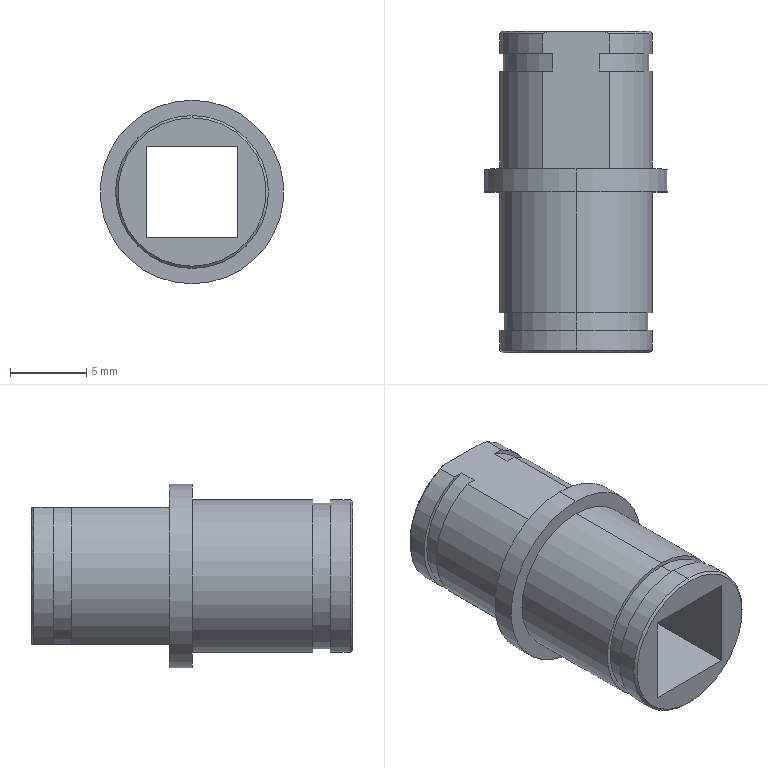Part | NX | features BREP 1 | 1 solid | 34 faces | box 12 x 21 x 12 mm | volume 902.734 mm3 | plane 16 | cylinder 14 | cone 4 | commonest cylinder face diameters 10 x8 9.5 x4 12 x2
STEP:
#1=CARTESIAN_POINT('',(0.,0.15,-5.));
#2=VERTEX_POINT('',#1);
#3=CARTESIAN_POINT('',(0.,0.,-4.85));
#4=VERTEX_POINT('',#3);
#5=CARTESIAN_POINT('',(0.,0.,-4.85));
#6=DIRECTION('',(0.,0.7071,-0.7071));
#7=VECTOR('',#6,1000.);
#8=LINE('',#5,#7);
#9=EDGE_CURVE('',#2,#4,#8,.F.);
#10=ORIENTED_EDGE('',*,*,#9,.T.);
#11=CARTESIAN_POINT('',(0.,0.,4.85));
#12=VERTEX_POINT('',#11);
#13=CARTESIAN_POINT('',(0.,0.,0.));
#14=DIRECTION('',(0.,-1.,0.));
#15=DIRECTION('',(0.,0.,1.));
#16=AXIS2_PLACEMENT_3D('',#13,#14,#15);
#17=CIRCLE('',#16,4.85);
#18=EDGE_CURVE('',#12,#4,#17,.T.);
#19=ORIENTED_EDGE('',*,*,#18,.F.);
#20=CARTESIAN_POINT('',(0.,0.15,5.));
#21=VERTEX_POINT('',#20);
#22=CARTESIAN_POINT('',(0.,0.,4.85));
#23=DIRECTION('',(0.,0.7071,0.7071));
#24=VECTOR('',#23,1000.);
#25=LINE('',#22,#24);
#26=EDGE_CURVE('',#21,#12,#25,.F.);
#27=ORIENTED_EDGE('',*,*,#26,.F.);
#28=CARTESIAN_POINT('',(0.,0.15,0.));
#29=DIRECTION('',(0.,1.,0.));
#30=DIRECTION('',(0.,0.,1.));
#31=AXIS2_PLACEMENT_3D('',#28,#29,#30);
#32=CIRCLE('',#31,5.);
#33=EDGE_CURVE('',#2,#21,#32,.T.);
#34=ORIENTED_EDGE('',*,*,#33,.F.);
#35=EDGE_LOOP('',(#10,#19,#27,#34));
#36=FACE_BOUND('',#35,.T.);
#37=CARTESIAN_POINT('',(0.,0.,0.));
#38=DIRECTION('',(0.,1.,0.));
#39=DIRECTION('',(0.,0.,1.));
#40=AXIS2_PLACEMENT_3D('',#37,#38,#39);
#41=CONICAL_SURFACE('',#40,4.85,0.7854);
#42=ADVANCED_FACE('',(#36),#41,.T.);
#43=CARTESIAN_POINT('',(1.809,21.,-4.5));
#44=VERTEX_POINT('',#43);
#45=CARTESIAN_POINT('',(2.179,20.85,-4.5));
#46=VERTEX_POINT('',#45);
#47=CARTESIAN_POINT('',(1.809,21.,-4.5));
#48=CARTESIAN_POINT('',(1.934,20.953,-4.5));
#49=CARTESIAN_POINT('',(2.057,20.903,-4.5));
#50=CARTESIAN_POINT('',(2.179,20.85,-4.5));
#51=B_SPLINE_CURVE_WITH_KNOTS('',3,(#47,#48,#49,#50),.UNSPECIFIED.,.F.,.F.,(4,4),(0.,0.0003997),.UNSPECIFIED.);
#52=EDGE_CURVE('',#44,#46,#51,.T.);
#53=ORIENTED_EDGE('',*,*,#52,.F.);
#54=CARTESIAN_POINT('',(1.809,21.,4.5));
#55=VERTEX_POINT('',#54);
#56=CARTESIAN_POINT('',(0.,21.,0.));
#57=DIRECTION('',(0.,1.,0.));
#58=DIRECTION('',(0.,0.,-1.));
#59=AXIS2_PLACEMENT_3D('',#56,#57,#58);
#60=CIRCLE('',#59,4.85);
#61=EDGE_CURVE('',#55,#44,#60,.T.);
#62=ORIENTED_EDGE('',*,*,#61,.F.);
#63=CARTESIAN_POINT('',(2.179,20.85,4.5));
#64=VERTEX_POINT('',#63);
#65=CARTESIAN_POINT('',(2.179,20.85,4.5));
#66=CARTESIAN_POINT('',(2.057,20.903,4.5));
#67=CARTESIAN_POINT('',(1.934,20.953,4.5));
#68=CARTESIAN_POINT('',(1.809,21.,4.5));
#69=B_SPLINE_CURVE_WITH_KNOTS('',3,(#65,#66,#67,#68),.UNSPECIFIED.,.F.,.F.,(4,4),(0.,0.0003997),.UNSPECIFIED.);
#70=EDGE_CURVE('',#64,#55,#69,.T.);
#71=ORIENTED_EDGE('',*,*,#70,.F.);
#72=CARTESIAN_POINT('',(0.,20.85,0.));
#73=DIRECTION('',(0.,-1.,0.));
#74=DIRECTION('',(0.,0.,-1.));
#75=AXIS2_PLACEMENT_3D('',#72,#73,#74);
#76=CIRCLE('',#75,5.);
#77=EDGE_CURVE('',#46,#64,#76,.T.);
#78=ORIENTED_EDGE('',*,*,#77,.F.);
#79=EDGE_LOOP('',(#53,#62,#71,#78));
#80=FACE_BOUND('',#79,.T.);
#81=CARTESIAN_POINT('',(0.,20.85,0.));
#82=DIRECTION('',(0.,-1.,0.));
#83=DIRECTION('',(0.,0.,-1.));
#84=AXIS2_PLACEMENT_3D('',#81,#82,#83);
#85=CONICAL_SURFACE('',#84,5.,0.7854);
#86=ADVANCED_FACE('',(#80),#85,.T.);
#87=CARTESIAN_POINT('',(-1.809,21.,4.5));
#88=VERTEX_POINT('',#87);
#89=CARTESIAN_POINT('',(-2.179,20.85,4.5));
#90=VERTEX_POINT('',#89);
#91=CARTESIAN_POINT('',(-1.809,21.,4.5));
#92=CARTESIAN_POINT('',(-1.934,20.953,4.5));
#93=CARTESIAN_POINT('',(-2.057,20.903,4.5));
#94=CARTESIAN_POINT('',(-2.179,20.85,4.5));
#95=B_SPLINE_CURVE_WITH_KNOTS('',3,(#91,#92,#93,#94),.UNSPECIFIED.,.F.,.F.,(4,4),(0.,0.0003997),.UNSPECIFIED.);
#96=EDGE_CURVE('',#88,#90,#95,.T.);
#97=ORIENTED_EDGE('',*,*,#96,.F.);
#98=CARTESIAN_POINT('',(-1.809,21.,-4.5));
#99=VERTEX_POINT('',#98);
#100=CARTESIAN_POINT('',(0.,21.,0.));
#101=DIRECTION('',(0.,1.,0.));
#102=DIRECTION('',(0.,0.,-1.));
#103=AXIS2_PLACEMENT_3D('',#100,#101,#102);
#104=CIRCLE('',#103,4.85);
#105=EDGE_CURVE('',#99,#88,#104,.T.);
#106=ORIENTED_EDGE('',*,*,#105,.F.);
#107=CARTESIAN_POINT('',(-2.179,20.85,-4.5));
#108=VERTEX_POINT('',#107);
#109=CARTESIAN_POINT('',(-2.179,20.85,-4.5));
#110=CARTESIAN_POINT('',(-2.057,20.903,-4.5));
#111=CARTESIAN_POINT('',(-1.934,20.953,-4.5));
#112=CARTESIAN_POINT('',(-1.809,21.,-4.5));
#113=B_SPLINE_CURVE_WITH_KNOTS('',3,(#109,#110,#111,#112),.UNSPECIFIED.,.F.,.F.,(4,4),(0.,0.0003997),.UNSPECIFIED.);
#114=EDGE_CURVE('',#108,#99,#113,.T.);
#115=ORIENTED_EDGE('',*,*,#114,.F.);
#116=CARTESIAN_POINT('',(0.,20.85,0.));
#117=DIRECTION('',(0.,-1.,0.));
#118=DIRECTION('',(0.,0.,-1.));
#119=AXIS2_PLACEMENT_3D('',#116,#117,#118);
#120=CIRCLE('',#119,5.);
#121=EDGE_CURVE('',#90,#108,#120,.T.);
#122=ORIENTED_EDGE('',*,*,#121,.F.);
#123=EDGE_LOOP('',(#97,#106,#115,#122));
#124=FACE_BOUND('',#123,.T.);
#125=CARTESIAN_POINT('',(0.,20.85,0.));
#126=DIRECTION('',(0.,-1.,0.));
#127=DIRECTION('',(0.,0.,-1.));
#128=AXIS2_PLACEMENT_3D('',#125,#126,#127);
#129=CONICAL_SURFACE('',#128,5.,0.7854);
#130=ADVANCED_FACE('',(#124),#129,.T.);
#131=CARTESIAN_POINT('',(-2.179,19.55,-4.5));
#132=VERTEX_POINT('',#131);
#133=CARTESIAN_POINT('',(-2.179,7.37,-4.5));
#134=DIRECTION('',(0.,1.,0.));
#135=VECTOR('',#134,1000.);
#136=LINE('',#133,#135);
#137=EDGE_CURVE('',#132,#108,#136,.T.);
#138=ORIENTED_EDGE('',*,*,#137,.T.);
#139=ORIENTED_EDGE('',*,*,#114,.T.);
#140=CARTESIAN_POINT('',(2.179,21.,-4.5));
#141=DIRECTION('',(1.,0.,0.));
#142=VECTOR('',#141,1000.);
#143=LINE('',#140,#142);
#144=EDGE_CURVE('',#99,#44,#143,.T.);
#145=ORIENTED_EDGE('',*,*,#144,.T.);
#146=ORIENTED_EDGE('',*,*,#52,.T.);
#147=CARTESIAN_POINT('',(2.179,19.55,-4.5));
#148=VERTEX_POINT('',#147);
#149=CARTESIAN_POINT('',(2.179,7.37,-4.5));
#150=DIRECTION('',(0.,1.,0.));
#151=VECTOR('',#150,1000.);
#152=LINE('',#149,#151);
#153=EDGE_CURVE('',#148,#46,#152,.T.);
#154=ORIENTED_EDGE('',*,*,#153,.F.);
#155=CARTESIAN_POINT('',(1.521,19.55,-4.5));
#156=VERTEX_POINT('',#155);
#157=CARTESIAN_POINT('',(0.,19.55,-4.5));
#158=DIRECTION('',(1.,0.,0.));
#159=VECTOR('',#158,1000.);
#160=LINE('',#157,#159);
#161=EDGE_CURVE('',#156,#148,#160,.T.);
#162=ORIENTED_EDGE('',*,*,#161,.F.);
#163=CARTESIAN_POINT('',(1.521,18.4,-4.5));
#164=VERTEX_POINT('',#163);
#165=CARTESIAN_POINT('',(1.521,19.55,-4.5));
#166=DIRECTION('',(0.,1.,0.));
#167=VECTOR('',#166,1000.);
#168=LINE('',#165,#167);
#169=EDGE_CURVE('',#164,#156,#168,.T.);
#170=ORIENTED_EDGE('',*,*,#169,.F.);
#171=CARTESIAN_POINT('',(2.179,18.4,-4.5));
#172=VERTEX_POINT('',#171);
#173=CARTESIAN_POINT('',(0.,18.4,-4.5));
#174=DIRECTION('',(1.,0.,0.));
#175=VECTOR('',#174,1000.);
#176=LINE('',#173,#175);
#177=EDGE_CURVE('',#164,#172,#176,.T.);
#178=ORIENTED_EDGE('',*,*,#177,.T.);
#179=CARTESIAN_POINT('',(2.179,12.,-4.5));
#180=VERTEX_POINT('',#179);
#181=CARTESIAN_POINT('',(2.179,7.37,-4.5));
#182=DIRECTION('',(0.,1.,0.));
#183=VECTOR('',#182,1000.);
#184=LINE('',#181,#183);
#185=EDGE_CURVE('',#180,#172,#184,.T.);
#186=ORIENTED_EDGE('',*,*,#185,.F.);
#187=CARTESIAN_POINT('',(-2.179,12.,-4.5));
#188=VERTEX_POINT('',#187);
#189=CARTESIAN_POINT('',(2.179,12.,-4.5));
#190=DIRECTION('',(1.,0.,0.));
#191=VECTOR('',#190,1000.);
#192=LINE('',#189,#191);
#193=EDGE_CURVE('',#188,#180,#192,.T.);
#194=ORIENTED_EDGE('',*,*,#193,.F.);
#195=CARTESIAN_POINT('',(-2.179,18.4,-4.5));
#196=VERTEX_POINT('',#195);
#197=CARTESIAN_POINT('',(-2.179,7.37,-4.5));
#198=DIRECTION('',(0.,1.,0.));
#199=VECTOR('',#198,1000.);
#200=LINE('',#197,#199);
#201=EDGE_CURVE('',#188,#196,#200,.T.);
#202=ORIENTED_EDGE('',*,*,#201,.T.);
#203=CARTESIAN_POINT('',(-1.521,18.4,-4.5));
#204=VERTEX_POINT('',#203);
#205=CARTESIAN_POINT('',(0.,18.4,-4.5));
#206=DIRECTION('',(1.,0.,0.));
#207=VECTOR('',#206,1000.);
#208=LINE('',#205,#207);
#209=EDGE_CURVE('',#196,#204,#208,.T.);
#210=ORIENTED_EDGE('',*,*,#209,.T.);
#211=CARTESIAN_POINT('',(-1.521,19.55,-4.5));
#212=VERTEX_POINT('',#211);
#213=CARTESIAN_POINT('',(-1.521,19.55,-4.5));
#214=DIRECTION('',(0.,-1.,0.));
#215=VECTOR('',#214,1000.);
#216=LINE('',#213,#215);
#217=EDGE_CURVE('',#212,#204,#216,.T.);
#218=ORIENTED_EDGE('',*,*,#217,.F.);
#219=CARTESIAN_POINT('',(0.,19.55,-4.5));
#220=DIRECTION('',(1.,0.,0.));
#221=VECTOR('',#220,1000.);
#222=LINE('',#219,#221);
#223=EDGE_CURVE('',#132,#212,#222,.T.);
#224=ORIENTED_EDGE('',*,*,#223,.F.);
#225=EDGE_LOOP('',(#138,#139,#145,#146,#154,#162,#170,#178,#186,#194,#202,#210,#218,#224));
#226=FACE_BOUND('',#225,.T.);
#227=CARTESIAN_POINT('',(2.179,7.37,-4.5));
#228=DIRECTION('',(0.,0.,1.));
#229=DIRECTION('',(1.,0.,0.));
#230=AXIS2_PLACEMENT_3D('',#227,#228,#229);
#231=PLANE('',#230);
#232=ADVANCED_FACE('',(#226),#231,.F.);
#233=CARTESIAN_POINT('',(2.179,21.,4.5));
#234=DIRECTION('',(-1.,0.,0.));
#235=VECTOR('',#234,1000.);
#236=LINE('',#233,#235);
#237=EDGE_CURVE('',#55,#88,#236,.T.);
#238=ORIENTED_EDGE('',*,*,#237,.T.);
#239=ORIENTED_EDGE('',*,*,#96,.T.);
#240=CARTESIAN_POINT('',(-2.179,19.55,4.5));
#241=VERTEX_POINT('',#240);
#242=CARTESIAN_POINT('',(-2.179,7.37,4.5));
#243=DIRECTION('',(0.,1.,0.));
#244=VECTOR('',#243,1000.);
#245=LINE('',#242,#244);
#246=EDGE_CURVE('',#241,#90,#245,.T.);
#247=ORIENTED_EDGE('',*,*,#246,.F.);
#248=CARTESIAN_POINT('',(-1.521,19.55,4.5));
#249=VERTEX_POINT('',#248);
#250=CARTESIAN_POINT('',(0.,19.55,4.5));
#251=DIRECTION('',(-1.,0.,0.));
#252=VECTOR('',#251,1000.);
#253=LINE('',#250,#252);
#254=EDGE_CURVE('',#249,#241,#253,.T.);
#255=ORIENTED_EDGE('',*,*,#254,.F.);
#256=CARTESIAN_POINT('',(-1.521,18.4,4.5));
#257=VERTEX_POINT('',#256);
#258=CARTESIAN_POINT('',(-1.521,19.55,4.5));
#259=DIRECTION('',(0.,1.,0.));
#260=VECTOR('',#259,1000.);
#261=LINE('',#258,#260);
#262=EDGE_CURVE('',#257,#249,#261,.T.);
#263=ORIENTED_EDGE('',*,*,#262,.F.);
#264=CARTESIAN_POINT('',(-2.179,18.4,4.5));
#265=VERTEX_POINT('',#264);
#266=CARTESIAN_POINT('',(0.,18.4,4.5));
#267=DIRECTION('',(-1.,0.,0.));
#268=VECTOR('',#267,1000.);
#269=LINE('',#266,#268);
#270=EDGE_CURVE('',#257,#265,#269,.T.);
#271=ORIENTED_EDGE('',*,*,#270,.T.);
#272=CARTESIAN_POINT('',(-2.179,12.,4.5));
#273=VERTEX_POINT('',#272);
#274=CARTESIAN_POINT('',(-2.179,7.37,4.5));
#275=DIRECTION('',(0.,1.,0.));
#276=VECTOR('',#275,1000.);
#277=LINE('',#274,#276);
#278=EDGE_CURVE('',#273,#265,#277,.T.);
#279=ORIENTED_EDGE('',*,*,#278,.F.);
#280=CARTESIAN_POINT('',(2.179,12.,4.5));
#281=VERTEX_POINT('',#280);
#282=CARTESIAN_POINT('',(2.179,12.,4.5));
#283=DIRECTION('',(-1.,0.,0.));
#284=VECTOR('',#283,1000.);
#285=LINE('',#282,#284);
#286=EDGE_CURVE('',#281,#273,#285,.T.);
#287=ORIENTED_EDGE('',*,*,#286,.F.);
#288=CARTESIAN_POINT('',(2.179,18.4,4.5));
#289=VERTEX_POINT('',#288);
#290=CARTESIAN_POINT('',(2.179,7.37,4.5));
#291=DIRECTION('',(0.,1.,0.));
#292=VECTOR('',#291,1000.);
#293=LINE('',#290,#292);
#294=EDGE_CURVE('',#281,#289,#293,.T.);
#295=ORIENTED_EDGE('',*,*,#294,.T.);
#296=CARTESIAN_POINT('',(1.521,18.4,4.5));
#297=VERTEX_POINT('',#296);
#298=CARTESIAN_POINT('',(0.,18.4,4.5));
#299=DIRECTION('',(-1.,0.,0.));
#300=VECTOR('',#299,1000.);
#301=LINE('',#298,#300);
#302=EDGE_CURVE('',#289,#297,#301,.T.);
#303=ORIENTED_EDGE('',*,*,#302,.T.);
#304=CARTESIAN_POINT('',(1.521,19.55,4.5));
#305=VERTEX_POINT('',#304);
#306=CARTESIAN_POINT('',(1.521,19.55,4.5));
#307=DIRECTION('',(0.,-1.,0.));
#308=VECTOR('',#307,1000.);
#309=LINE('',#306,#308);
#310=EDGE_CURVE('',#305,#297,#309,.T.);
#311=ORIENTED_EDGE('',*,*,#310,.F.);
#312=CARTESIAN_POINT('',(2.179,19.55,4.5));
#313=VERTEX_POINT('',#312);
#314=CARTESIAN_POINT('',(0.,19.55,4.5));
#315=DIRECTION('',(-1.,0.,0.));
#316=VECTOR('',#315,1000.);
#317=LINE('',#314,#316);
#318=EDGE_CURVE('',#313,#305,#317,.T.);
#319=ORIENTED_EDGE('',*,*,#318,.F.);
#320=CARTESIAN_POINT('',(2.179,7.37,4.5));
#321=DIRECTION('',(0.,1.,0.));
#322=VECTOR('',#321,1000.);
#323=LINE('',#320,#322);
#324=EDGE_CURVE('',#313,#64,#323,.T.);
#325=ORIENTED_EDGE('',*,*,#324,.T.);
#326=ORIENTED_EDGE('',*,*,#70,.T.);
#327=EDGE_LOOP('',(#238,#239,#247,#255,#263,#271,#279,#287,#295,#303,#311,#319,#325,#326));
#328=FACE_BOUND('',#327,.T.);
#329=CARTESIAN_POINT('',(2.179,7.37,4.5));
#330=DIRECTION('',(0.,0.,-1.));
#331=DIRECTION('',(-1.,0.,0.));
#332=AXIS2_PLACEMENT_3D('',#329,#330,#331);
#333=PLANE('',#332);
#334=ADVANCED_FACE('',(#328),#333,.F.);
#335=CARTESIAN_POINT('',(0.,18.4,0.));
#336=DIRECTION('',(0.,1.,0.));
#337=DIRECTION('',(0.,0.,1.));
#338=AXIS2_PLACEMENT_3D('',#335,#336,#337);
#339=CIRCLE('',#338,4.75);
#340=EDGE_CURVE('',#297,#164,#339,.T.);
#341=ORIENTED_EDGE('',*,*,#340,.T.);
#342=ORIENTED_EDGE('',*,*,#169,.T.);
#343=CARTESIAN_POINT('',(0.,19.55,0.));
#344=DIRECTION('',(0.,1.,0.));
#345=DIRECTION('',(0.,0.,1.));
#346=AXIS2_PLACEMENT_3D('',#343,#344,#345);
#347=CIRCLE('',#346,4.75);
#348=EDGE_CURVE('',#305,#156,#347,.T.);
#349=ORIENTED_EDGE('',*,*,#348,.F.);
#350=ORIENTED_EDGE('',*,*,#310,.T.);
#351=EDGE_LOOP('',(#341,#342,#349,#350));
#352=FACE_BOUND('',#351,.T.);
#353=CARTESIAN_POINT('',(0.,19.55,0.));
#354=DIRECTION('',(0.,-1.,0.));
#355=DIRECTION('',(0.,0.,-1.));
#356=AXIS2_PLACEMENT_3D('',#353,#354,#355);
#357=CYLINDRICAL_SURFACE('',#356,4.75);
#358=ADVANCED_FACE('',(#352),#357,.T.);
#359=ORIENTED_EDGE('',*,*,#177,.F.);
#360=ORIENTED_EDGE('',*,*,#340,.F.);
#361=ORIENTED_EDGE('',*,*,#302,.F.);
#362=CARTESIAN_POINT('',(0.,18.4,0.));
#363=DIRECTION('',(0.,1.,0.));
#364=DIRECTION('',(0.,0.,1.));
#365=AXIS2_PLACEMENT_3D('',#362,#363,#364);
#366=CIRCLE('',#365,5.);
#367=EDGE_CURVE('',#289,#172,#366,.T.);
#368=ORIENTED_EDGE('',*,*,#367,.T.);
#369=EDGE_LOOP('',(#359,#360,#361,#368));
#370=FACE_BOUND('',#369,.T.);
#371=CARTESIAN_POINT('',(0.,18.4,0.));
#372=DIRECTION('',(0.,1.,0.));
#373=DIRECTION('',(0.,0.,1.));
#374=AXIS2_PLACEMENT_3D('',#371,#372,#373);
#375=PLANE('',#374);
#376=ADVANCED_FACE('',(#370),#375,.T.);
#377=ORIENTED_EDGE('',*,*,#348,.T.);
#378=ORIENTED_EDGE('',*,*,#161,.T.);
#379=CARTESIAN_POINT('',(0.,19.55,0.));
#380=DIRECTION('',(0.,1.,0.));
#381=DIRECTION('',(0.,0.,1.));
#382=AXIS2_PLACEMENT_3D('',#379,#380,#381);
#383=CIRCLE('',#382,5.);
#384=EDGE_CURVE('',#313,#148,#383,.T.);
#385=ORIENTED_EDGE('',*,*,#384,.F.);
#386=ORIENTED_EDGE('',*,*,#318,.T.);
#387=EDGE_LOOP('',(#377,#378,#385,#386));
#388=FACE_BOUND('',#387,.T.);
#389=CARTESIAN_POINT('',(0.,19.55,0.));
#390=DIRECTION('',(0.,1.,0.));
#391=DIRECTION('',(0.,0.,1.));
#392=AXIS2_PLACEMENT_3D('',#389,#390,#391);
#393=PLANE('',#392);
#394=ADVANCED_FACE('',(#388),#393,.F.);
#395=CARTESIAN_POINT('',(3.,21.,3.));
#396=VERTEX_POINT('',#395);
#397=CARTESIAN_POINT('',(3.,0.,3.));
#398=VERTEX_POINT('',#397);
#399=CARTESIAN_POINT('',(3.,40.,3.));
#400=DIRECTION('',(0.,-1.,0.));
#401=VECTOR('',#400,1000.);
#402=LINE('',#399,#401);
#403=EDGE_CURVE('',#396,#398,#402,.T.);
#404=ORIENTED_EDGE('',*,*,#403,.T.);
#405=CARTESIAN_POINT('',(-3.,0.,3.));
#406=VERTEX_POINT('',#405);
#407=CARTESIAN_POINT('',(-3.,0.,3.));
#408=DIRECTION('',(-1.,0.,0.));
#409=VECTOR('',#408,1000.);
#410=LINE('',#407,#409);
#411=EDGE_CURVE('',#398,#406,#410,.T.);
#412=ORIENTED_EDGE('',*,*,#411,.T.);
#413=CARTESIAN_POINT('',(-3.,21.,3.));
#414=VERTEX_POINT('',#413);
#415=CARTESIAN_POINT('',(-3.,40.,3.));
#416=DIRECTION('',(0.,-1.,0.));
#417=VECTOR('',#416,1000.);
#418=LINE('',#415,#417);
#419=EDGE_CURVE('',#414,#406,#418,.T.);
#420=ORIENTED_EDGE('',*,*,#419,.F.);
#421=CARTESIAN_POINT('',(-5.,21.,3.));
#422=DIRECTION('',(-1.,0.,0.));
#423=VECTOR('',#422,1000.);
#424=LINE('',#421,#423);
#425=EDGE_CURVE('',#396,#414,#424,.T.);
#426=ORIENTED_EDGE('',*,*,#425,.F.);
#427=EDGE_LOOP('',(#404,#412,#420,#426));
#428=FACE_BOUND('',#427,.T.);
#429=CARTESIAN_POINT('',(-3.,40.,3.));
#430=DIRECTION('',(0.,0.,1.));
#431=DIRECTION('',(1.,0.,0.));
#432=AXIS2_PLACEMENT_3D('',#429,#430,#431);
#433=PLANE('',#432);
#434=ADVANCED_FACE('',(#428),#433,.F.);
#435=ORIENTED_EDGE('',*,*,#419,.T.);
#436=CARTESIAN_POINT('',(-3.,0.,-3.));
#437=VERTEX_POINT('',#436);
#438=CARTESIAN_POINT('',(-3.,0.,-3.));
#439=DIRECTION('',(0.,0.,-1.));
#440=VECTOR('',#439,1000.);
#441=LINE('',#438,#440);
#442=EDGE_CURVE('',#406,#437,#441,.T.);
#443=ORIENTED_EDGE('',*,*,#442,.T.);
#444=CARTESIAN_POINT('',(-3.,21.,-3.));
#445=VERTEX_POINT('',#444);
#446=CARTESIAN_POINT('',(-3.,40.,-3.));
#447=DIRECTION('',(0.,-1.,0.));
#448=VECTOR('',#447,1000.);
#449=LINE('',#446,#448);
#450=EDGE_CURVE('',#445,#437,#449,.T.);
#451=ORIENTED_EDGE('',*,*,#450,.F.);
#452=CARTESIAN_POINT('',(-3.,21.,0.));
#453=DIRECTION('',(0.,0.,-1.));
#454=VECTOR('',#453,1000.);
#455=LINE('',#452,#454);
#456=EDGE_CURVE('',#414,#445,#455,.T.);
#457=ORIENTED_EDGE('',*,*,#456,.F.);
#458=EDGE_LOOP('',(#435,#443,#451,#457));
#459=FACE_BOUND('',#458,.T.);
#460=CARTESIAN_POINT('',(-3.,40.,-3.));
#461=DIRECTION('',(-1.,0.,0.));
#462=DIRECTION('',(0.,0.,1.));
#463=AXIS2_PLACEMENT_3D('',#460,#461,#462);
#464=PLANE('',#463);
#465=ADVANCED_FACE('',(#459),#464,.F.);
#466=ORIENTED_EDGE('',*,*,#450,.T.);
#467=CARTESIAN_POINT('',(3.,0.,-3.));
#468=VERTEX_POINT('',#467);
#469=CARTESIAN_POINT('',(-3.,0.,-3.));
#470=DIRECTION('',(1.,0.,0.));
#471=VECTOR('',#470,1000.);
#472=LINE('',#469,#471);
#473=EDGE_CURVE('',#437,#468,#472,.T.);
#474=ORIENTED_EDGE('',*,*,#473,.T.);
#475=CARTESIAN_POINT('',(3.,21.,-3.));
#476=VERTEX_POINT('',#475);
#477=CARTESIAN_POINT('',(3.,40.,-3.));
#478=DIRECTION('',(0.,-1.,0.));
#479=VECTOR('',#478,1000.);
#480=LINE('',#477,#479);
#481=EDGE_CURVE('',#476,#468,#480,.T.);
#482=ORIENTED_EDGE('',*,*,#481,.F.);
#483=CARTESIAN_POINT('',(-5.,21.,-3.));
#484=DIRECTION('',(1.,0.,0.));
#485=VECTOR('',#484,1000.);
#486=LINE('',#483,#485);
#487=EDGE_CURVE('',#445,#476,#486,.T.);
#488=ORIENTED_EDGE('',*,*,#487,.F.);
#489=EDGE_LOOP('',(#466,#474,#482,#488));
#490=FACE_BOUND('',#489,.T.);
#491=CARTESIAN_POINT('',(-3.,40.,-3.));
#492=DIRECTION('',(0.,0.,-1.));
#493=DIRECTION('',(-1.,0.,0.));
#494=AXIS2_PLACEMENT_3D('',#491,#492,#493);
#495=PLANE('',#494);
#496=ADVANCED_FACE('',(#490),#495,.F.);
#497=ORIENTED_EDGE('',*,*,#481,.T.);
#498=CARTESIAN_POINT('',(3.,0.,-3.));
#499=DIRECTION('',(0.,0.,1.));
#500=VECTOR('',#499,1000.);
#501=LINE('',#498,#500);
#502=EDGE_CURVE('',#468,#398,#501,.T.);
#503=ORIENTED_EDGE('',*,*,#502,.T.);
#504=ORIENTED_EDGE('',*,*,#403,.F.);
#505=CARTESIAN_POINT('',(3.,21.,0.));
#506=DIRECTION('',(0.,0.,1.));
#507=VECTOR('',#506,1000.);
#508=LINE('',#505,#507);
#509=EDGE_CURVE('',#476,#396,#508,.T.);
#510=ORIENTED_EDGE('',*,*,#509,.F.);
#511=EDGE_LOOP('',(#497,#503,#504,#510));
#512=FACE_BOUND('',#511,.T.);
#513=CARTESIAN_POINT('',(3.,40.,-3.));
#514=DIRECTION('',(1.,0.,0.));
#515=DIRECTION('',(0.,0.,-1.));
#516=AXIS2_PLACEMENT_3D('',#513,#514,#515);
#517=PLANE('',#516);
#518=ADVANCED_FACE('',(#512),#517,.F.);
#519=ORIENTED_EDGE('',*,*,#144,.F.);
#520=ORIENTED_EDGE('',*,*,#105,.T.);
#521=ORIENTED_EDGE('',*,*,#237,.F.);
#522=ORIENTED_EDGE('',*,*,#61,.T.);
#523=EDGE_LOOP('',(#519,#520,#521,#522));
#524=FACE_BOUND('',#523,.T.);
#525=ORIENTED_EDGE('',*,*,#487,.T.);
#526=ORIENTED_EDGE('',*,*,#509,.T.);
#527=ORIENTED_EDGE('',*,*,#425,.T.);
#528=ORIENTED_EDGE('',*,*,#456,.T.);
#529=EDGE_LOOP('',(#525,#526,#527,#528));
#530=FACE_BOUND('',#529,.T.);
#531=CARTESIAN_POINT('',(-5.,21.,0.));
#532=DIRECTION('',(0.,-1.,0.));
#533=DIRECTION('',(0.,0.,-1.));
#534=AXIS2_PLACEMENT_3D('',#531,#532,#533);
#535=PLANE('',#534);
#536=ADVANCED_FACE('',(#524,#530),#535,.F.);
#537=ORIENTED_EDGE('',*,*,#153,.T.);
#538=ORIENTED_EDGE('',*,*,#77,.T.);
#539=ORIENTED_EDGE('',*,*,#324,.F.);
#540=ORIENTED_EDGE('',*,*,#384,.T.);
#541=EDGE_LOOP('',(#537,#538,#539,#540));
#542=FACE_BOUND('',#541,.T.);
#543=CARTESIAN_POINT('',(0.,0.,0.));
#544=DIRECTION('',(0.,-1.,0.));
#545=DIRECTION('',(0.,0.,-1.));
#546=AXIS2_PLACEMENT_3D('',#543,#544,#545);
#547=CYLINDRICAL_SURFACE('',#546,5.);
#548=ADVANCED_FACE('',(#542),#547,.T.);
#549=CARTESIAN_POINT('',(0.,12.,-6.));
#550=VERTEX_POINT('',#549);
#551=CARTESIAN_POINT('',(0.,12.,6.));
#552=VERTEX_POINT('',#551);
#553=CARTESIAN_POINT('',(0.,12.,0.));
#554=DIRECTION('',(0.,-1.,0.));
#555=DIRECTION('',(0.,0.,-1.));
#556=AXIS2_PLACEMENT_3D('',#553,#554,#555);
#557=CIRCLE('',#556,6.);
#558=EDGE_CURVE('',#550,#552,#557,.T.);
#559=ORIENTED_EDGE('',*,*,#558,.F.);
#560=CARTESIAN_POINT('',(0.,12.,0.));
#561=DIRECTION('',(0.,-1.,0.));
#562=DIRECTION('',(0.,0.,-1.));
#563=AXIS2_PLACEMENT_3D('',#560,#561,#562);
#564=CIRCLE('',#563,6.);
#565=EDGE_CURVE('',#552,#550,#564,.T.);
#566=ORIENTED_EDGE('',*,*,#565,.F.);
#567=EDGE_LOOP('',(#559,#566));
#568=FACE_BOUND('',#567,.T.);
#569=CARTESIAN_POINT('',(0.,12.,0.));
#570=DIRECTION('',(0.,-1.,0.));
#571=DIRECTION('',(0.,0.,-1.));
#572=AXIS2_PLACEMENT_3D('',#569,#570,#571);
#573=CIRCLE('',#572,5.);
#574=EDGE_CURVE('',#273,#188,#573,.T.);
#575=ORIENTED_EDGE('',*,*,#574,.T.);
#576=ORIENTED_EDGE('',*,*,#193,.T.);
#577=CARTESIAN_POINT('',(0.,12.,0.));
#578=DIRECTION('',(0.,-1.,0.));
#579=DIRECTION('',(0.,0.,-1.));
#580=AXIS2_PLACEMENT_3D('',#577,#578,#579);
#581=CIRCLE('',#580,5.);
#582=EDGE_CURVE('',#180,#281,#581,.T.);
#583=ORIENTED_EDGE('',*,*,#582,.T.);
#584=ORIENTED_EDGE('',*,*,#286,.T.);
#585=EDGE_LOOP('',(#575,#576,#583,#584));
#586=FACE_BOUND('',#585,.T.);
#587=CARTESIAN_POINT('',(-6.,12.,0.));
#588=DIRECTION('',(0.,-1.,0.));
#589=DIRECTION('',(0.,0.,-1.));
#590=AXIS2_PLACEMENT_3D('',#587,#588,#589);
#591=PLANE('',#590);
#592=ADVANCED_FACE('',(#568,#586),#591,.F.);
#593=CARTESIAN_POINT('',(0.,10.5,6.));
#594=VERTEX_POINT('',#593);
#595=CARTESIAN_POINT('',(0.,0.,6.));
#596=DIRECTION('',(0.,-1.,0.));
#597=VECTOR('',#596,1000.);
#598=LINE('',#595,#597);
#599=EDGE_CURVE('',#552,#594,#598,.T.);
#600=ORIENTED_EDGE('',*,*,#599,.F.);
#601=ORIENTED_EDGE('',*,*,#565,.T.);
#602=CARTESIAN_POINT('',(0.,10.5,-6.));
#603=VERTEX_POINT('',#602);
#604=CARTESIAN_POINT('',(0.,0.,-6.));
#605=DIRECTION('',(0.,-1.,0.));
#606=VECTOR('',#605,1000.);
#607=LINE('',#604,#606);
#608=EDGE_CURVE('',#550,#603,#607,.T.);
#609=ORIENTED_EDGE('',*,*,#608,.T.);
#610=CARTESIAN_POINT('',(0.,10.5,0.));
#611=DIRECTION('',(0.,-1.,0.));
#612=DIRECTION('',(0.,0.,-1.));
#613=AXIS2_PLACEMENT_3D('',#610,#611,#612);
#614=CIRCLE('',#613,6.);
#615=EDGE_CURVE('',#594,#603,#614,.T.);
#616=ORIENTED_EDGE('',*,*,#615,.F.);
#617=EDGE_LOOP('',(#600,#601,#609,#616));
#618=FACE_BOUND('',#617,.T.);
#619=CARTESIAN_POINT('',(0.,0.,0.));
#620=DIRECTION('',(0.,-1.,0.));
#621=DIRECTION('',(0.,0.,-1.));
#622=AXIS2_PLACEMENT_3D('',#619,#620,#621);
#623=CYLINDRICAL_SURFACE('',#622,6.);
#624=ADVANCED_FACE('',(#618),#623,.T.);
#625=CARTESIAN_POINT('',(0.,10.5,0.));
#626=DIRECTION('',(0.,-1.,0.));
#627=DIRECTION('',(0.,0.,-1.));
#628=AXIS2_PLACEMENT_3D('',#625,#626,#627);
#629=CIRCLE('',#628,6.);
#630=EDGE_CURVE('',#603,#594,#629,.T.);
#631=ORIENTED_EDGE('',*,*,#630,.T.);
#632=ORIENTED_EDGE('',*,*,#615,.T.);
#633=EDGE_LOOP('',(#631,#632));
#634=FACE_BOUND('',#633,.T.);
#635=CARTESIAN_POINT('',(0.,10.5,-5.));
#636=VERTEX_POINT('',#635);
#637=CARTESIAN_POINT('',(0.,10.5,5.));
#638=VERTEX_POINT('',#637);
#639=CARTESIAN_POINT('',(0.,10.5,0.));
#640=DIRECTION('',(0.,-1.,0.));
#641=DIRECTION('',(0.,0.,-1.));
#642=AXIS2_PLACEMENT_3D('',#639,#640,#641);
#643=CIRCLE('',#642,5.);
#644=EDGE_CURVE('',#636,#638,#643,.T.);
#645=ORIENTED_EDGE('',*,*,#644,.F.);
#646=CARTESIAN_POINT('',(0.,10.5,0.));
#647=DIRECTION('',(0.,-1.,0.));
#648=DIRECTION('',(0.,0.,-1.));
#649=AXIS2_PLACEMENT_3D('',#646,#647,#648);
#650=CIRCLE('',#649,5.);
#651=EDGE_CURVE('',#638,#636,#650,.T.);
#652=ORIENTED_EDGE('',*,*,#651,.F.);
#653=EDGE_LOOP('',(#645,#652));
#654=FACE_BOUND('',#653,.T.);
#655=CARTESIAN_POINT('',(-5.,10.5,0.));
#656=DIRECTION('',(0.,1.,0.));
#657=DIRECTION('',(0.,0.,1.));
#658=AXIS2_PLACEMENT_3D('',#655,#656,#657);
#659=PLANE('',#658);
#660=ADVANCED_FACE('',(#634,#654),#659,.F.);
#661=CARTESIAN_POINT('',(0.,2.6,5.));
#662=VERTEX_POINT('',#661);
#663=CARTESIAN_POINT('',(0.,0.,5.));
#664=DIRECTION('',(0.,-1.,0.));
#665=VECTOR('',#664,1000.);
#666=LINE('',#663,#665);
#667=EDGE_CURVE('',#638,#662,#666,.T.);
#668=ORIENTED_EDGE('',*,*,#667,.F.);
#669=ORIENTED_EDGE('',*,*,#651,.T.);
#670=CARTESIAN_POINT('',(0.,2.6,-5.));
#671=VERTEX_POINT('',#670);
#672=CARTESIAN_POINT('',(0.,0.,-5.));
#673=DIRECTION('',(0.,-1.,0.));
#674=VECTOR('',#673,1000.);
#675=LINE('',#672,#674);
#676=EDGE_CURVE('',#636,#671,#675,.T.);
#677=ORIENTED_EDGE('',*,*,#676,.T.);
#678=CARTESIAN_POINT('',(0.,2.6,0.));
#679=DIRECTION('',(0.,-1.,0.));
#680=DIRECTION('',(0.,0.,-1.));
#681=AXIS2_PLACEMENT_3D('',#678,#679,#680);
#682=CIRCLE('',#681,5.);
#683=EDGE_CURVE('',#662,#671,#682,.T.);
#684=ORIENTED_EDGE('',*,*,#683,.F.);
#685=EDGE_LOOP('',(#668,#669,#677,#684));
#686=FACE_BOUND('',#685,.T.);
#687=CARTESIAN_POINT('',(0.,0.,0.));
#688=DIRECTION('',(0.,-1.,0.));
#689=DIRECTION('',(0.,0.,-1.));
#690=AXIS2_PLACEMENT_3D('',#687,#688,#689);
#691=CYLINDRICAL_SURFACE('',#690,5.);
#692=ADVANCED_FACE('',(#686),#691,.T.);
#693=CARTESIAN_POINT('',(0.,2.6,0.));
#694=DIRECTION('',(0.,-1.,0.));
#695=DIRECTION('',(0.,0.,-1.));
#696=AXIS2_PLACEMENT_3D('',#693,#694,#695);
#697=CIRCLE('',#696,5.);
#698=EDGE_CURVE('',#671,#662,#697,.T.);
#699=ORIENTED_EDGE('',*,*,#698,.T.);
#700=ORIENTED_EDGE('',*,*,#683,.T.);
#701=EDGE_LOOP('',(#699,#700));
#702=FACE_BOUND('',#701,.T.);
#703=CARTESIAN_POINT('',(0.,2.6,-4.75));
#704=VERTEX_POINT('',#703);
#705=CARTESIAN_POINT('',(0.,2.6,4.75));
#706=VERTEX_POINT('',#705);
#707=CARTESIAN_POINT('',(0.,2.6,0.));
#708=DIRECTION('',(0.,-1.,0.));
#709=DIRECTION('',(0.,0.,-1.));
#710=AXIS2_PLACEMENT_3D('',#707,#708,#709);
#711=CIRCLE('',#710,4.75);
#712=EDGE_CURVE('',#704,#706,#711,.T.);
#713=ORIENTED_EDGE('',*,*,#712,.F.);
#714=CARTESIAN_POINT('',(0.,2.6,0.));
#715=DIRECTION('',(0.,-1.,0.));
#716=DIRECTION('',(0.,0.,-1.));
#717=AXIS2_PLACEMENT_3D('',#714,#715,#716);
#718=CIRCLE('',#717,4.75);
#719=EDGE_CURVE('',#706,#704,#718,.T.);
#720=ORIENTED_EDGE('',*,*,#719,.F.);
#721=EDGE_LOOP('',(#713,#720));
#722=FACE_BOUND('',#721,.T.);
#723=CARTESIAN_POINT('',(-4.75,2.6,0.));
#724=DIRECTION('',(0.,1.,0.));
#725=DIRECTION('',(0.,0.,1.));
#726=AXIS2_PLACEMENT_3D('',#723,#724,#725);
#727=PLANE('',#726);
#728=ADVANCED_FACE('',(#702,#722),#727,.F.);
#729=CARTESIAN_POINT('',(0.,1.45,4.75));
#730=VERTEX_POINT('',#729);
#731=CARTESIAN_POINT('',(0.,0.,4.75));
#732=DIRECTION('',(0.,-1.,0.));
#733=VECTOR('',#732,1000.);
#734=LINE('',#731,#733);
#735=EDGE_CURVE('',#706,#730,#734,.T.);
#736=ORIENTED_EDGE('',*,*,#735,.F.);
#737=ORIENTED_EDGE('',*,*,#719,.T.);
#738=CARTESIAN_POINT('',(0.,1.45,-4.75));
#739=VERTEX_POINT('',#738);
#740=CARTESIAN_POINT('',(0.,0.,-4.75));
#741=DIRECTION('',(0.,-1.,0.));
#742=VECTOR('',#741,1000.);
#743=LINE('',#740,#742);
#744=EDGE_CURVE('',#704,#739,#743,.T.);
#745=ORIENTED_EDGE('',*,*,#744,.T.);
#746=CARTESIAN_POINT('',(0.,1.45,0.));
#747=DIRECTION('',(0.,-1.,0.));
#748=DIRECTION('',(0.,0.,-1.));
#749=AXIS2_PLACEMENT_3D('',#746,#747,#748);
#750=CIRCLE('',#749,4.75);
#751=EDGE_CURVE('',#730,#739,#750,.T.);
#752=ORIENTED_EDGE('',*,*,#751,.F.);
#753=EDGE_LOOP('',(#736,#737,#745,#752));
#754=FACE_BOUND('',#753,.T.);
#755=CARTESIAN_POINT('',(0.,0.,0.));
#756=DIRECTION('',(0.,-1.,0.));
#757=DIRECTION('',(0.,0.,-1.));
#758=AXIS2_PLACEMENT_3D('',#755,#756,#757);
#759=CYLINDRICAL_SURFACE('',#758,4.75);
#760=ADVANCED_FACE('',(#754),#759,.T.);
#761=CARTESIAN_POINT('',(0.,1.45,0.));
#762=DIRECTION('',(0.,-1.,0.));
#763=DIRECTION('',(0.,0.,-1.));
#764=AXIS2_PLACEMENT_3D('',#761,#762,#763);
#765=CIRCLE('',#764,4.75);
#766=EDGE_CURVE('',#739,#730,#765,.T.);
#767=ORIENTED_EDGE('',*,*,#766,.T.);
#768=ORIENTED_EDGE('',*,*,#751,.T.);
#769=EDGE_LOOP('',(#767,#768));
#770=FACE_BOUND('',#769,.T.);
#771=CARTESIAN_POINT('',(0.,1.45,-5.));
#772=VERTEX_POINT('',#771);
#773=CARTESIAN_POINT('',(0.,1.45,5.));
#774=VERTEX_POINT('',#773);
#775=CARTESIAN_POINT('',(0.,1.45,0.));
#776=DIRECTION('',(0.,-1.,0.));
#777=DIRECTION('',(0.,0.,-1.));
#778=AXIS2_PLACEMENT_3D('',#775,#776,#777);
#779=CIRCLE('',#778,5.);
#780=EDGE_CURVE('',#772,#774,#779,.T.);
#781=ORIENTED_EDGE('',*,*,#780,.F.);
#782=CARTESIAN_POINT('',(0.,1.45,0.));
#783=DIRECTION('',(0.,-1.,0.));
#784=DIRECTION('',(0.,0.,-1.));
#785=AXIS2_PLACEMENT_3D('',#782,#783,#784);
#786=CIRCLE('',#785,5.);
#787=EDGE_CURVE('',#774,#772,#786,.T.);
#788=ORIENTED_EDGE('',*,*,#787,.F.);
#789=EDGE_LOOP('',(#781,#788));
#790=FACE_BOUND('',#789,.T.);
#791=CARTESIAN_POINT('',(-5.,1.45,0.));
#792=DIRECTION('',(0.,-1.,0.));
#793=DIRECTION('',(0.,0.,-1.));
#794=AXIS2_PLACEMENT_3D('',#791,#792,#793);
#795=PLANE('',#794);
#796=ADVANCED_FACE('',(#770,#790),#795,.F.);
#797=CARTESIAN_POINT('',(0.,0.,5.));
#798=DIRECTION('',(0.,-1.,0.));
#799=VECTOR('',#798,1000.);
#800=LINE('',#797,#799);
#801=EDGE_CURVE('',#774,#21,#800,.T.);
#802=ORIENTED_EDGE('',*,*,#801,.F.);
#803=ORIENTED_EDGE('',*,*,#787,.T.);
#804=CARTESIAN_POINT('',(0.,0.,-5.));
#805=DIRECTION('',(0.,-1.,0.));
#806=VECTOR('',#805,1000.);
#807=LINE('',#804,#806);
#808=EDGE_CURVE('',#772,#2,#807,.T.);
#809=ORIENTED_EDGE('',*,*,#808,.T.);
#810=ORIENTED_EDGE('',*,*,#33,.T.);
#811=EDGE_LOOP('',(#802,#803,#809,#810));
#812=FACE_BOUND('',#811,.T.);
#813=CARTESIAN_POINT('',(0.,0.,0.));
#814=DIRECTION('',(0.,-1.,0.));
#815=DIRECTION('',(0.,0.,-1.));
#816=AXIS2_PLACEMENT_3D('',#813,#814,#815);
#817=CYLINDRICAL_SURFACE('',#816,5.);
#818=ADVANCED_FACE('',(#812),#817,.T.);
#819=ORIENTED_EDGE('',*,*,#411,.F.);
#820=ORIENTED_EDGE('',*,*,#502,.F.);
#821=ORIENTED_EDGE('',*,*,#473,.F.);
#822=ORIENTED_EDGE('',*,*,#442,.F.);
#823=EDGE_LOOP('',(#819,#820,#821,#822));
#824=FACE_BOUND('',#823,.T.);
#825=ORIENTED_EDGE('',*,*,#18,.T.);
#826=CARTESIAN_POINT('',(0.,0.,0.));
#827=DIRECTION('',(0.,-1.,0.));
#828=DIRECTION('',(0.,0.,1.));
#829=AXIS2_PLACEMENT_3D('',#826,#827,#828);
#830=CIRCLE('',#829,4.85);
#831=EDGE_CURVE('',#4,#12,#830,.T.);
#832=ORIENTED_EDGE('',*,*,#831,.T.);
#833=EDGE_LOOP('',(#825,#832));
#834=FACE_BOUND('',#833,.T.);
#835=CARTESIAN_POINT('',(0.,0.,0.));
#836=DIRECTION('',(0.,1.,0.));
#837=DIRECTION('',(0.,0.,1.));
#838=AXIS2_PLACEMENT_3D('',#835,#836,#837);
#839=PLANE('',#838);
#840=ADVANCED_FACE('',(#824,#834),#839,.F.);
#841=ORIENTED_EDGE('',*,*,#582,.F.);
#842=ORIENTED_EDGE('',*,*,#185,.T.);
#843=ORIENTED_EDGE('',*,*,#367,.F.);
#844=ORIENTED_EDGE('',*,*,#294,.F.);
#845=EDGE_LOOP('',(#841,#842,#843,#844));
#846=FACE_BOUND('',#845,.T.);
#847=CARTESIAN_POINT('',(0.,0.,0.));
#848=DIRECTION('',(0.,-1.,0.));
#849=DIRECTION('',(0.,0.,-1.));
#850=AXIS2_PLACEMENT_3D('',#847,#848,#849);
#851=CYLINDRICAL_SURFACE('',#850,5.);
#852=ADVANCED_FACE('',(#846),#851,.T.);
#853=CARTESIAN_POINT('',(0.,19.55,0.));
#854=DIRECTION('',(0.,1.,0.));
#855=DIRECTION('',(0.,0.,1.));
#856=AXIS2_PLACEMENT_3D('',#853,#854,#855);
#857=CIRCLE('',#856,4.75);
#858=EDGE_CURVE('',#212,#249,#857,.T.);
#859=ORIENTED_EDGE('',*,*,#858,.F.);
#860=ORIENTED_EDGE('',*,*,#217,.T.);
#861=CARTESIAN_POINT('',(0.,18.4,0.));
#862=DIRECTION('',(0.,1.,0.));
#863=DIRECTION('',(0.,0.,1.));
#864=AXIS2_PLACEMENT_3D('',#861,#862,#863);
#865=CIRCLE('',#864,4.75);
#866=EDGE_CURVE('',#204,#257,#865,.T.);
#867=ORIENTED_EDGE('',*,*,#866,.T.);
#868=ORIENTED_EDGE('',*,*,#262,.T.);
#869=EDGE_LOOP('',(#859,#860,#867,#868));
#870=FACE_BOUND('',#869,.T.);
#871=CARTESIAN_POINT('',(0.,19.55,0.));
#872=DIRECTION('',(0.,-1.,0.));
#873=DIRECTION('',(0.,0.,-1.));
#874=AXIS2_PLACEMENT_3D('',#871,#872,#873);
#875=CYLINDRICAL_SURFACE('',#874,4.75);
#876=ADVANCED_FACE('',(#870),#875,.T.);
#877=ORIENTED_EDGE('',*,*,#209,.F.);
#878=CARTESIAN_POINT('',(0.,18.4,0.));
#879=DIRECTION('',(0.,1.,0.));
#880=DIRECTION('',(0.,0.,1.));
#881=AXIS2_PLACEMENT_3D('',#878,#879,#880);
#882=CIRCLE('',#881,5.);
#883=EDGE_CURVE('',#196,#265,#882,.T.);
#884=ORIENTED_EDGE('',*,*,#883,.T.);
#885=ORIENTED_EDGE('',*,*,#270,.F.);
#886=ORIENTED_EDGE('',*,*,#866,.F.);
#887=EDGE_LOOP('',(#877,#884,#885,#886));
#888=FACE_BOUND('',#887,.T.);
#889=CARTESIAN_POINT('',(0.,18.4,0.));
#890=DIRECTION('',(0.,1.,0.));
#891=DIRECTION('',(0.,0.,1.));
#892=AXIS2_PLACEMENT_3D('',#889,#890,#891);
#893=PLANE('',#892);
#894=ADVANCED_FACE('',(#888),#893,.T.);
#895=CARTESIAN_POINT('',(0.,19.55,0.));
#896=DIRECTION('',(0.,1.,0.));
#897=DIRECTION('',(0.,0.,1.));
#898=AXIS2_PLACEMENT_3D('',#895,#896,#897);
#899=CIRCLE('',#898,5.);
#900=EDGE_CURVE('',#132,#241,#899,.T.);
#901=ORIENTED_EDGE('',*,*,#900,.F.);
#902=ORIENTED_EDGE('',*,*,#223,.T.);
#903=ORIENTED_EDGE('',*,*,#858,.T.);
#904=ORIENTED_EDGE('',*,*,#254,.T.);
#905=EDGE_LOOP('',(#901,#902,#903,#904));
#906=FACE_BOUND('',#905,.T.);
#907=CARTESIAN_POINT('',(0.,19.55,0.));
#908=DIRECTION('',(0.,1.,0.));
#909=DIRECTION('',(0.,0.,1.));
#910=AXIS2_PLACEMENT_3D('',#907,#908,#909);
#911=PLANE('',#910);
#912=ADVANCED_FACE('',(#906),#911,.F.);
#913=ORIENTED_EDGE('',*,*,#246,.T.);
#914=ORIENTED_EDGE('',*,*,#121,.T.);
#915=ORIENTED_EDGE('',*,*,#137,.F.);
#916=ORIENTED_EDGE('',*,*,#900,.T.);
#917=EDGE_LOOP('',(#913,#914,#915,#916));
#918=FACE_BOUND('',#917,.T.);
#919=CARTESIAN_POINT('',(0.,0.,0.));
#920=DIRECTION('',(0.,-1.,0.));
#921=DIRECTION('',(0.,0.,-1.));
#922=AXIS2_PLACEMENT_3D('',#919,#920,#921);
#923=CYLINDRICAL_SURFACE('',#922,5.);
#924=ADVANCED_FACE('',(#918),#923,.T.);
#925=ORIENTED_EDGE('',*,*,#883,.F.);
#926=ORIENTED_EDGE('',*,*,#201,.F.);
#927=ORIENTED_EDGE('',*,*,#574,.F.);
#928=ORIENTED_EDGE('',*,*,#278,.T.);
#929=EDGE_LOOP('',(#925,#926,#927,#928));
#930=FACE_BOUND('',#929,.T.);
#931=CARTESIAN_POINT('',(0.,0.,0.));
#932=DIRECTION('',(0.,-1.,0.));
#933=DIRECTION('',(0.,0.,-1.));
#934=AXIS2_PLACEMENT_3D('',#931,#932,#933);
#935=CYLINDRICAL_SURFACE('',#934,5.);
#936=ADVANCED_FACE('',(#930),#935,.T.);
#937=ORIENTED_EDGE('',*,*,#780,.T.);
#938=ORIENTED_EDGE('',*,*,#801,.T.);
#939=CARTESIAN_POINT('',(0.,0.15,0.));
#940=DIRECTION('',(0.,1.,0.));
#941=DIRECTION('',(0.,0.,1.));
#942=AXIS2_PLACEMENT_3D('',#939,#940,#941);
#943=CIRCLE('',#942,5.);
#944=EDGE_CURVE('',#21,#2,#943,.T.);
#945=ORIENTED_EDGE('',*,*,#944,.T.);
#946=ORIENTED_EDGE('',*,*,#808,.F.);
#947=EDGE_LOOP('',(#937,#938,#945,#946));
#948=FACE_BOUND('',#947,.T.);
#949=CARTESIAN_POINT('',(0.,0.,0.));
#950=DIRECTION('',(0.,-1.,0.));
#951=DIRECTION('',(0.,0.,-1.));
#952=AXIS2_PLACEMENT_3D('',#949,#950,#951);
#953=CYLINDRICAL_SURFACE('',#952,5.);
#954=ADVANCED_FACE('',(#948),#953,.T.);
#955=ORIENTED_EDGE('',*,*,#712,.T.);
#956=ORIENTED_EDGE('',*,*,#735,.T.);
#957=ORIENTED_EDGE('',*,*,#766,.F.);
#958=ORIENTED_EDGE('',*,*,#744,.F.);
#959=EDGE_LOOP('',(#955,#956,#957,#958));
#960=FACE_BOUND('',#959,.T.);
#961=CARTESIAN_POINT('',(0.,0.,0.));
#962=DIRECTION('',(0.,-1.,0.));
#963=DIRECTION('',(0.,0.,-1.));
#964=AXIS2_PLACEMENT_3D('',#961,#962,#963);
#965=CYLINDRICAL_SURFACE('',#964,4.75);
#966=ADVANCED_FACE('',(#960),#965,.T.);
#967=ORIENTED_EDGE('',*,*,#644,.T.);
#968=ORIENTED_EDGE('',*,*,#667,.T.);
#969=ORIENTED_EDGE('',*,*,#698,.F.);
#970=ORIENTED_EDGE('',*,*,#676,.F.);
#971=EDGE_LOOP('',(#967,#968,#969,#970));
#972=FACE_BOUND('',#971,.T.);
#973=CARTESIAN_POINT('',(0.,0.,0.));
#974=DIRECTION('',(0.,-1.,0.));
#975=DIRECTION('',(0.,0.,-1.));
#976=AXIS2_PLACEMENT_3D('',#973,#974,#975);
#977=CYLINDRICAL_SURFACE('',#976,5.);
#978=ADVANCED_FACE('',(#972),#977,.T.);
#979=ORIENTED_EDGE('',*,*,#558,.T.);
#980=ORIENTED_EDGE('',*,*,#599,.T.);
#981=ORIENTED_EDGE('',*,*,#630,.F.);
#982=ORIENTED_EDGE('',*,*,#608,.F.);
#983=EDGE_LOOP('',(#979,#980,#981,#982));
#984=FACE_BOUND('',#983,.T.);
#985=CARTESIAN_POINT('',(0.,0.,0.));
#986=DIRECTION('',(0.,-1.,0.));
#987=DIRECTION('',(0.,0.,-1.));
#988=AXIS2_PLACEMENT_3D('',#985,#986,#987);
#989=CYLINDRICAL_SURFACE('',#988,6.);
#990=ADVANCED_FACE('',(#984),#989,.T.);
#991=ORIENTED_EDGE('',*,*,#831,.F.);
#992=ORIENTED_EDGE('',*,*,#9,.F.);
#993=ORIENTED_EDGE('',*,*,#944,.F.);
#994=ORIENTED_EDGE('',*,*,#26,.T.);
#995=EDGE_LOOP('',(#991,#992,#993,#994));
#996=FACE_BOUND('',#995,.T.);
#997=CARTESIAN_POINT('',(0.,0.,0.));
#998=DIRECTION('',(0.,1.,0.));
#999=DIRECTION('',(0.,0.,1.));
#1000=AXIS2_PLACEMENT_3D('',#997,#998,#999);
#1001=CONICAL_SURFACE('',#1000,4.85,0.7854);
#1002=ADVANCED_FACE('',(#996),#1001,.T.);
#1003=CLOSED_SHELL('',(#42,#86,#130,#232,#334,#358,#376,#394,#434,#465,#496,#518,#536,#548,#592,#624,#660,#692,#728,#760,#796,#818,#840,#852,#876,#894,#912,#924,#936,#954,#966,#978,#990,#1002));
#1004=MANIFOLD_SOLID_BREP('',#1003);
#1005=(LENGTH_UNIT()NAMED_UNIT(*)SI_UNIT(.MILLI.,.METRE.));
#1006=UNCERTAINTY_MEASURE_WITH_UNIT(LENGTH_MEASURE(0.00001),#1005,'','');
#1007=(NAMED_UNIT(*)PLANE_ANGLE_UNIT()SI_UNIT($,.RADIAN.));
#1008=(NAMED_UNIT(*)SI_UNIT($,.STERADIAN.)SOLID_ANGLE_UNIT());
#1009=(GEOMETRIC_REPRESENTATION_CONTEXT(3)GLOBAL_UNCERTAINTY_ASSIGNED_CONTEXT((#1006))GLOBAL_UNIT_ASSIGNED_CONTEXT((#1005,#1007,#1008))REPRESENTATION_CONTEXT('',''));
#1010=ADVANCED_BREP_SHAPE_REPRESENTATION('',(#1004),#1009);